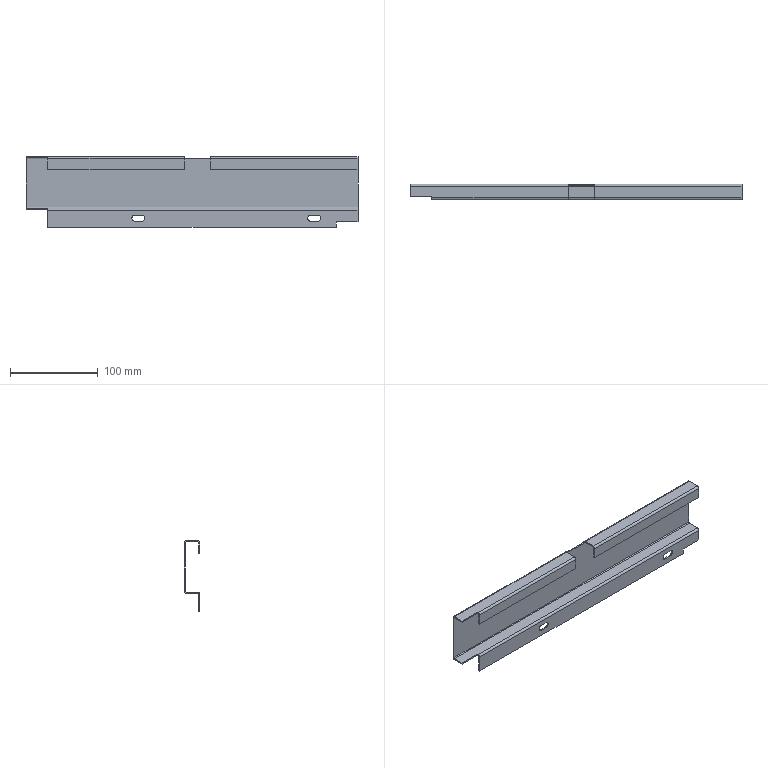Part | STEP file | 1 solid | 65 faces | box 378 x 18 x 80.5 mm | volume 66912 mm3 | plane 49 | cylinder 16 | commonest cylinder face diameters 2 x6 5 x6 7 x4